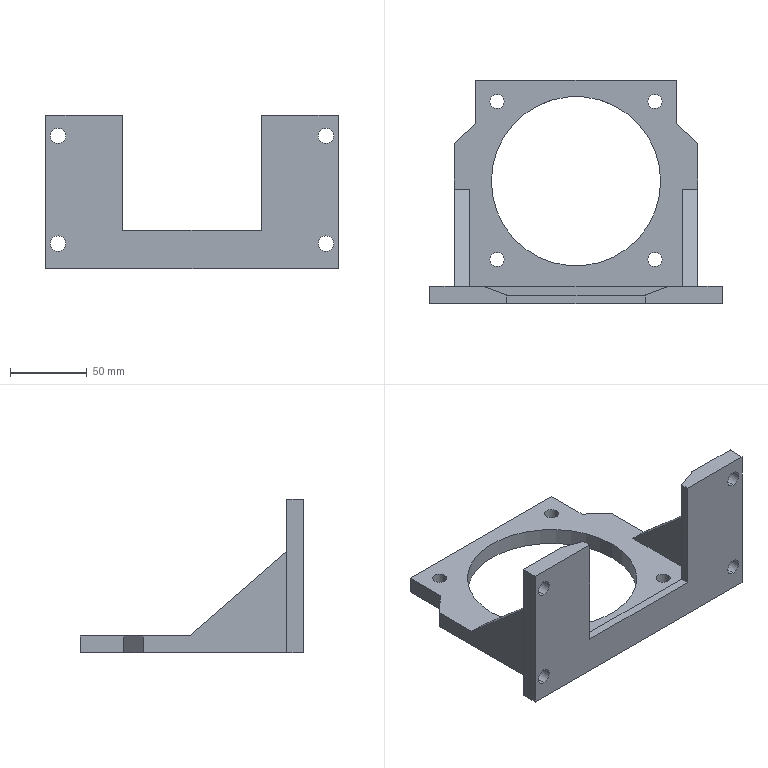Part | SolidWorks | features ICE 3, Extrusion 1, MirrorPattern 1 | 1 solid | 45 faces | box 190 x 145 x 100 mm | volume 268946 mm3 | plane 27 | cylinder 18 | commonest cylinder face diameters 9.2 x8 10 x8 110 x2
STEP:
#1=CARTESIAN_POINT('',(87.,-80.,85.957));
#2=VERTEX_POINT('',#1);
#3=CARTESIAN_POINT('',(87.,-80.,75.957));
#4=VERTEX_POINT('',#3);
#5=CARTESIAN_POINT('',(87.,-80.,80.957));
#6=DIRECTION('',(0.,-1.,0.));
#7=DIRECTION('',(0.,0.,1.));
#8=AXIS2_PLACEMENT_3D('',#5,#6,#7);
#9=CIRCLE('',#8,5.);
#10=EDGE_CURVE('',#2,#4,#9,.T.);
#11=ORIENTED_EDGE('',*,*,#10,.T.);
#12=CARTESIAN_POINT('',(87.,-69.,75.957));
#13=VERTEX_POINT('',#12);
#14=CARTESIAN_POINT('',(87.,-80.,75.957));
#15=DIRECTION('',(0.,1.,0.));
#16=VECTOR('',#15,1000.);
#17=LINE('',#14,#16);
#18=EDGE_CURVE('',#4,#13,#17,.T.);
#19=ORIENTED_EDGE('',*,*,#18,.T.);
#20=CARTESIAN_POINT('',(87.,-69.,85.957));
#21=VERTEX_POINT('',#20);
#22=CARTESIAN_POINT('',(87.,-69.,80.957));
#23=DIRECTION('',(0.,-1.,0.));
#24=DIRECTION('',(0.,0.,1.));
#25=AXIS2_PLACEMENT_3D('',#22,#23,#24);
#26=CIRCLE('',#25,5.);
#27=EDGE_CURVE('',#21,#13,#26,.T.);
#28=ORIENTED_EDGE('',*,*,#27,.F.);
#29=CARTESIAN_POINT('',(87.,-80.,85.957));
#30=DIRECTION('',(0.,1.,0.));
#31=VECTOR('',#30,1000.);
#32=LINE('',#29,#31);
#33=EDGE_CURVE('',#2,#21,#32,.T.);
#34=ORIENTED_EDGE('',*,*,#33,.F.);
#35=EDGE_LOOP('',(#11,#19,#28,#34));
#36=FACE_OUTER_BOUND('',#35,.T.);
#37=CARTESIAN_POINT('',(87.,-80.,80.957));
#38=DIRECTION('',(0.,1.,0.));
#39=DIRECTION('',(0.,0.,1.));
#40=AXIS2_PLACEMENT_3D('',#37,#38,#39);
#41=CYLINDRICAL_SURFACE('',#40,5.);
#42=ADVANCED_FACE('',(#36),#41,.F.);
#43=CARTESIAN_POINT('',(87.,-80.,15.957));
#44=VERTEX_POINT('',#43);
#45=CARTESIAN_POINT('',(87.,-80.,5.957));
#46=VERTEX_POINT('',#45);
#47=CARTESIAN_POINT('',(87.,-80.,10.957));
#48=DIRECTION('',(0.,-1.,0.));
#49=DIRECTION('',(0.,0.,1.));
#50=AXIS2_PLACEMENT_3D('',#47,#48,#49);
#51=CIRCLE('',#50,5.);
#52=EDGE_CURVE('',#44,#46,#51,.T.);
#53=ORIENTED_EDGE('',*,*,#52,.T.);
#54=CARTESIAN_POINT('',(87.,-69.,5.957));
#55=VERTEX_POINT('',#54);
#56=CARTESIAN_POINT('',(87.,-80.,5.957));
#57=DIRECTION('',(0.,1.,0.));
#58=VECTOR('',#57,1000.);
#59=LINE('',#56,#58);
#60=EDGE_CURVE('',#46,#55,#59,.T.);
#61=ORIENTED_EDGE('',*,*,#60,.T.);
#62=CARTESIAN_POINT('',(87.,-69.,15.957));
#63=VERTEX_POINT('',#62);
#64=CARTESIAN_POINT('',(87.,-69.,10.957));
#65=DIRECTION('',(0.,-1.,0.));
#66=DIRECTION('',(0.,0.,1.));
#67=AXIS2_PLACEMENT_3D('',#64,#65,#66);
#68=CIRCLE('',#67,5.);
#69=EDGE_CURVE('',#63,#55,#68,.T.);
#70=ORIENTED_EDGE('',*,*,#69,.F.);
#71=CARTESIAN_POINT('',(87.,-80.,15.957));
#72=DIRECTION('',(0.,1.,0.));
#73=VECTOR('',#72,1000.);
#74=LINE('',#71,#73);
#75=EDGE_CURVE('',#44,#63,#74,.T.);
#76=ORIENTED_EDGE('',*,*,#75,.F.);
#77=EDGE_LOOP('',(#53,#61,#70,#76));
#78=FACE_OUTER_BOUND('',#77,.T.);
#79=CARTESIAN_POINT('',(87.,-80.,10.957));
#80=DIRECTION('',(0.,1.,0.));
#81=DIRECTION('',(0.,0.,1.));
#82=AXIS2_PLACEMENT_3D('',#79,#80,#81);
#83=CYLINDRICAL_SURFACE('',#82,5.);
#84=ADVANCED_FACE('',(#78),#83,.F.);
#85=CARTESIAN_POINT('',(-87.,-80.,15.957));
#86=VERTEX_POINT('',#85);
#87=CARTESIAN_POINT('',(-87.,-80.,5.957));
#88=VERTEX_POINT('',#87);
#89=CARTESIAN_POINT('',(-87.,-80.,10.957));
#90=DIRECTION('',(0.,-1.,0.));
#91=DIRECTION('',(0.,0.,-1.));
#92=AXIS2_PLACEMENT_3D('',#89,#90,#91);
#93=CIRCLE('',#92,5.);
#94=EDGE_CURVE('',#86,#88,#93,.T.);
#95=ORIENTED_EDGE('',*,*,#94,.T.);
#96=CARTESIAN_POINT('',(-87.,-69.,5.957));
#97=VERTEX_POINT('',#96);
#98=CARTESIAN_POINT('',(-87.,-80.,5.957));
#99=DIRECTION('',(0.,1.,0.));
#100=VECTOR('',#99,1000.);
#101=LINE('',#98,#100);
#102=EDGE_CURVE('',#88,#97,#101,.T.);
#103=ORIENTED_EDGE('',*,*,#102,.T.);
#104=CARTESIAN_POINT('',(-87.,-69.,15.957));
#105=VERTEX_POINT('',#104);
#106=CARTESIAN_POINT('',(-87.,-69.,10.957));
#107=DIRECTION('',(0.,-1.,0.));
#108=DIRECTION('',(0.,0.,-1.));
#109=AXIS2_PLACEMENT_3D('',#106,#107,#108);
#110=CIRCLE('',#109,5.);
#111=EDGE_CURVE('',#105,#97,#110,.T.);
#112=ORIENTED_EDGE('',*,*,#111,.F.);
#113=CARTESIAN_POINT('',(-87.,-80.,15.957));
#114=DIRECTION('',(0.,1.,0.));
#115=VECTOR('',#114,1000.);
#116=LINE('',#113,#115);
#117=EDGE_CURVE('',#86,#105,#116,.T.);
#118=ORIENTED_EDGE('',*,*,#117,.F.);
#119=EDGE_LOOP('',(#95,#103,#112,#118));
#120=FACE_OUTER_BOUND('',#119,.T.);
#121=CARTESIAN_POINT('',(-87.,-80.,10.957));
#122=DIRECTION('',(0.,1.,0.));
#123=DIRECTION('',(0.,0.,1.));
#124=AXIS2_PLACEMENT_3D('',#121,#122,#123);
#125=CYLINDRICAL_SURFACE('',#124,5.);
#126=ADVANCED_FACE('',(#120),#125,.F.);
#127=CARTESIAN_POINT('',(-87.,-80.,85.957));
#128=VERTEX_POINT('',#127);
#129=CARTESIAN_POINT('',(-87.,-80.,75.957));
#130=VERTEX_POINT('',#129);
#131=CARTESIAN_POINT('',(-87.,-80.,80.957));
#132=DIRECTION('',(0.,-1.,0.));
#133=DIRECTION('',(0.,0.,-1.));
#134=AXIS2_PLACEMENT_3D('',#131,#132,#133);
#135=CIRCLE('',#134,5.);
#136=EDGE_CURVE('',#128,#130,#135,.T.);
#137=ORIENTED_EDGE('',*,*,#136,.T.);
#138=CARTESIAN_POINT('',(-87.,-69.,75.957));
#139=VERTEX_POINT('',#138);
#140=CARTESIAN_POINT('',(-87.,-80.,75.957));
#141=DIRECTION('',(0.,1.,0.));
#142=VECTOR('',#141,1000.);
#143=LINE('',#140,#142);
#144=EDGE_CURVE('',#130,#139,#143,.T.);
#145=ORIENTED_EDGE('',*,*,#144,.T.);
#146=CARTESIAN_POINT('',(-87.,-69.,85.957));
#147=VERTEX_POINT('',#146);
#148=CARTESIAN_POINT('',(-87.,-69.,80.957));
#149=DIRECTION('',(0.,-1.,0.));
#150=DIRECTION('',(0.,0.,-1.));
#151=AXIS2_PLACEMENT_3D('',#148,#149,#150);
#152=CIRCLE('',#151,5.);
#153=EDGE_CURVE('',#147,#139,#152,.T.);
#154=ORIENTED_EDGE('',*,*,#153,.F.);
#155=CARTESIAN_POINT('',(-87.,-80.,85.957));
#156=DIRECTION('',(0.,1.,0.));
#157=VECTOR('',#156,1000.);
#158=LINE('',#155,#157);
#159=EDGE_CURVE('',#128,#147,#158,.T.);
#160=ORIENTED_EDGE('',*,*,#159,.F.);
#161=EDGE_LOOP('',(#137,#145,#154,#160));
#162=FACE_OUTER_BOUND('',#161,.T.);
#163=CARTESIAN_POINT('',(-87.,-80.,80.957));
#164=DIRECTION('',(0.,1.,0.));
#165=DIRECTION('',(0.,0.,1.));
#166=AXIS2_PLACEMENT_3D('',#163,#164,#165);
#167=CYLINDRICAL_SURFACE('',#166,5.);
#168=ADVANCED_FACE('',(#162),#167,.F.);
#169=CARTESIAN_POINT('',(-46.7,-51.3,5.5));
#170=VERTEX_POINT('',#169);
#171=CARTESIAN_POINT('',(-55.9,-51.3,5.5));
#172=VERTEX_POINT('',#171);
#173=CARTESIAN_POINT('',(-51.3,-51.3,5.5));
#174=DIRECTION('',(0.,0.,-1.));
#175=DIRECTION('',(1.,0.,0.));
#176=AXIS2_PLACEMENT_3D('',#173,#174,#175);
#177=CIRCLE('',#176,4.6);
#178=EDGE_CURVE('',#170,#172,#177,.T.);
#179=ORIENTED_EDGE('',*,*,#178,.F.);
#180=CARTESIAN_POINT('',(-46.7,-51.3,-5.5));
#181=VERTEX_POINT('',#180);
#182=CARTESIAN_POINT('',(-46.7,-51.3,5.5));
#183=DIRECTION('',(0.,0.,-1.));
#184=VECTOR('',#183,1000.);
#185=LINE('',#182,#184);
#186=EDGE_CURVE('',#170,#181,#185,.T.);
#187=ORIENTED_EDGE('',*,*,#186,.T.);
#188=CARTESIAN_POINT('',(-55.9,-51.3,-5.5));
#189=VERTEX_POINT('',#188);
#190=CARTESIAN_POINT('',(-51.3,-51.3,-5.5));
#191=DIRECTION('',(0.,0.,-1.));
#192=DIRECTION('',(1.,0.,0.));
#193=AXIS2_PLACEMENT_3D('',#190,#191,#192);
#194=CIRCLE('',#193,4.6);
#195=EDGE_CURVE('',#181,#189,#194,.T.);
#196=ORIENTED_EDGE('',*,*,#195,.T.);
#197=CARTESIAN_POINT('',(-55.9,-51.3,5.5));
#198=DIRECTION('',(0.,0.,-1.));
#199=VECTOR('',#198,1000.);
#200=LINE('',#197,#199);
#201=EDGE_CURVE('',#172,#189,#200,.T.);
#202=ORIENTED_EDGE('',*,*,#201,.F.);
#203=EDGE_LOOP('',(#179,#187,#196,#202));
#204=FACE_OUTER_BOUND('',#203,.T.);
#205=CARTESIAN_POINT('',(-51.3,-51.3,5.5));
#206=DIRECTION('',(0.,0.,-1.));
#207=DIRECTION('',(-1.,0.,0.));
#208=AXIS2_PLACEMENT_3D('',#205,#206,#207);
#209=CYLINDRICAL_SURFACE('',#208,4.6);
#210=ADVANCED_FACE('',(#204),#209,.F.);
#211=CARTESIAN_POINT('',(55.9,-51.3,5.5));
#212=VERTEX_POINT('',#211);
#213=CARTESIAN_POINT('',(46.7,-51.3,5.5));
#214=VERTEX_POINT('',#213);
#215=CARTESIAN_POINT('',(51.3,-51.3,5.5));
#216=DIRECTION('',(0.,0.,-1.));
#217=DIRECTION('',(1.,0.,0.));
#218=AXIS2_PLACEMENT_3D('',#215,#216,#217);
#219=CIRCLE('',#218,4.6);
#220=EDGE_CURVE('',#212,#214,#219,.T.);
#221=ORIENTED_EDGE('',*,*,#220,.F.);
#222=CARTESIAN_POINT('',(55.9,-51.3,-5.5));
#223=VERTEX_POINT('',#222);
#224=CARTESIAN_POINT('',(55.9,-51.3,5.5));
#225=DIRECTION('',(0.,0.,-1.));
#226=VECTOR('',#225,1000.);
#227=LINE('',#224,#226);
#228=EDGE_CURVE('',#212,#223,#227,.T.);
#229=ORIENTED_EDGE('',*,*,#228,.T.);
#230=CARTESIAN_POINT('',(46.7,-51.3,-5.5));
#231=VERTEX_POINT('',#230);
#232=CARTESIAN_POINT('',(51.3,-51.3,-5.5));
#233=DIRECTION('',(0.,0.,-1.));
#234=DIRECTION('',(1.,0.,0.));
#235=AXIS2_PLACEMENT_3D('',#232,#233,#234);
#236=CIRCLE('',#235,4.6);
#237=EDGE_CURVE('',#223,#231,#236,.T.);
#238=ORIENTED_EDGE('',*,*,#237,.T.);
#239=CARTESIAN_POINT('',(46.7,-51.3,5.5));
#240=DIRECTION('',(0.,0.,-1.));
#241=VECTOR('',#240,1000.);
#242=LINE('',#239,#241);
#243=EDGE_CURVE('',#214,#231,#242,.T.);
#244=ORIENTED_EDGE('',*,*,#243,.F.);
#245=EDGE_LOOP('',(#221,#229,#238,#244));
#246=FACE_OUTER_BOUND('',#245,.T.);
#247=CARTESIAN_POINT('',(51.3,-51.3,5.5));
#248=DIRECTION('',(0.,0.,-1.));
#249=DIRECTION('',(-1.,0.,0.));
#250=AXIS2_PLACEMENT_3D('',#247,#248,#249);
#251=CYLINDRICAL_SURFACE('',#250,4.6);
#252=ADVANCED_FACE('',(#246),#251,.F.);
#253=CARTESIAN_POINT('',(46.7,51.3,5.5));
#254=VERTEX_POINT('',#253);
#255=CARTESIAN_POINT('',(55.9,51.3,5.5));
#256=VERTEX_POINT('',#255);
#257=CARTESIAN_POINT('',(51.3,51.3,5.5));
#258=DIRECTION('',(0.,0.,1.));
#259=DIRECTION('',(1.,0.,0.));
#260=AXIS2_PLACEMENT_3D('',#257,#258,#259);
#261=CIRCLE('',#260,4.6);
#262=EDGE_CURVE('',#254,#256,#261,.T.);
#263=ORIENTED_EDGE('',*,*,#262,.T.);
#264=CARTESIAN_POINT('',(55.9,51.3,-5.5));
#265=VERTEX_POINT('',#264);
#266=CARTESIAN_POINT('',(55.9,51.3,5.5));
#267=DIRECTION('',(0.,0.,-1.));
#268=VECTOR('',#267,1000.);
#269=LINE('',#266,#268);
#270=EDGE_CURVE('',#256,#265,#269,.T.);
#271=ORIENTED_EDGE('',*,*,#270,.T.);
#272=CARTESIAN_POINT('',(46.7,51.3,-5.5));
#273=VERTEX_POINT('',#272);
#274=CARTESIAN_POINT('',(51.3,51.3,-5.5));
#275=DIRECTION('',(0.,0.,1.));
#276=DIRECTION('',(1.,0.,0.));
#277=AXIS2_PLACEMENT_3D('',#274,#275,#276);
#278=CIRCLE('',#277,4.6);
#279=EDGE_CURVE('',#273,#265,#278,.T.);
#280=ORIENTED_EDGE('',*,*,#279,.F.);
#281=CARTESIAN_POINT('',(46.7,51.3,5.5));
#282=DIRECTION('',(0.,0.,-1.));
#283=VECTOR('',#282,1000.);
#284=LINE('',#281,#283);
#285=EDGE_CURVE('',#254,#273,#284,.T.);
#286=ORIENTED_EDGE('',*,*,#285,.F.);
#287=EDGE_LOOP('',(#263,#271,#280,#286));
#288=FACE_OUTER_BOUND('',#287,.T.);
#289=CARTESIAN_POINT('',(51.3,51.3,5.5));
#290=DIRECTION('',(0.,0.,-1.));
#291=DIRECTION('',(-1.,0.,0.));
#292=AXIS2_PLACEMENT_3D('',#289,#290,#291);
#293=CYLINDRICAL_SURFACE('',#292,4.6);
#294=ADVANCED_FACE('',(#288),#293,.F.);
#295=CARTESIAN_POINT('',(-55.9,51.3,5.5));
#296=VERTEX_POINT('',#295);
#297=CARTESIAN_POINT('',(-46.7,51.3,5.5));
#298=VERTEX_POINT('',#297);
#299=CARTESIAN_POINT('',(-51.3,51.3,5.5));
#300=DIRECTION('',(0.,0.,1.));
#301=DIRECTION('',(1.,0.,0.));
#302=AXIS2_PLACEMENT_3D('',#299,#300,#301);
#303=CIRCLE('',#302,4.6);
#304=EDGE_CURVE('',#296,#298,#303,.T.);
#305=ORIENTED_EDGE('',*,*,#304,.T.);
#306=CARTESIAN_POINT('',(-46.7,51.3,-5.5));
#307=VERTEX_POINT('',#306);
#308=CARTESIAN_POINT('',(-46.7,51.3,5.5));
#309=DIRECTION('',(0.,0.,-1.));
#310=VECTOR('',#309,1000.);
#311=LINE('',#308,#310);
#312=EDGE_CURVE('',#298,#307,#311,.T.);
#313=ORIENTED_EDGE('',*,*,#312,.T.);
#314=CARTESIAN_POINT('',(-55.9,51.3,-5.5));
#315=VERTEX_POINT('',#314);
#316=CARTESIAN_POINT('',(-51.3,51.3,-5.5));
#317=DIRECTION('',(0.,0.,1.));
#318=DIRECTION('',(1.,0.,0.));
#319=AXIS2_PLACEMENT_3D('',#316,#317,#318);
#320=CIRCLE('',#319,4.6);
#321=EDGE_CURVE('',#315,#307,#320,.T.);
#322=ORIENTED_EDGE('',*,*,#321,.F.);
#323=CARTESIAN_POINT('',(-55.9,51.3,5.5));
#324=DIRECTION('',(0.,0.,-1.));
#325=VECTOR('',#324,1000.);
#326=LINE('',#323,#325);
#327=EDGE_CURVE('',#296,#315,#326,.T.);
#328=ORIENTED_EDGE('',*,*,#327,.F.);
#329=EDGE_LOOP('',(#305,#313,#322,#328));
#330=FACE_OUTER_BOUND('',#329,.T.);
#331=CARTESIAN_POINT('',(-51.3,51.3,5.5));
#332=DIRECTION('',(0.,0.,-1.));
#333=DIRECTION('',(-1.,0.,0.));
#334=AXIS2_PLACEMENT_3D('',#331,#332,#333);
#335=CYLINDRICAL_SURFACE('',#334,4.6);
#336=ADVANCED_FACE('',(#330),#335,.F.);
#337=CARTESIAN_POINT('',(-55.,-0.5,5.5));
#338=VERTEX_POINT('',#337);
#339=CARTESIAN_POINT('',(55.,-0.5,5.5));
#340=VERTEX_POINT('',#339);
#341=CARTESIAN_POINT('',(0.,-0.5,5.5));
#342=DIRECTION('',(0.,0.,1.));
#343=DIRECTION('',(1.,0.,0.));
#344=AXIS2_PLACEMENT_3D('',#341,#342,#343);
#345=CIRCLE('',#344,55.);
#346=EDGE_CURVE('',#338,#340,#345,.T.);
#347=ORIENTED_EDGE('',*,*,#346,.T.);
#348=CARTESIAN_POINT('',(55.,-0.5,-5.5));
#349=VERTEX_POINT('',#348);
#350=CARTESIAN_POINT('',(55.,-0.5,5.5));
#351=DIRECTION('',(0.,0.,-1.));
#352=VECTOR('',#351,1000.);
#353=LINE('',#350,#352);
#354=EDGE_CURVE('',#340,#349,#353,.T.);
#355=ORIENTED_EDGE('',*,*,#354,.T.);
#356=CARTESIAN_POINT('',(-55.,-0.5,-5.5));
#357=VERTEX_POINT('',#356);
#358=CARTESIAN_POINT('',(0.,-0.5,-5.5));
#359=DIRECTION('',(0.,0.,1.));
#360=DIRECTION('',(1.,0.,0.));
#361=AXIS2_PLACEMENT_3D('',#358,#359,#360);
#362=CIRCLE('',#361,55.);
#363=EDGE_CURVE('',#357,#349,#362,.T.);
#364=ORIENTED_EDGE('',*,*,#363,.F.);
#365=CARTESIAN_POINT('',(-55.,-0.5,5.5));
#366=DIRECTION('',(0.,0.,-1.));
#367=VECTOR('',#366,1000.);
#368=LINE('',#365,#367);
#369=EDGE_CURVE('',#338,#357,#368,.T.);
#370=ORIENTED_EDGE('',*,*,#369,.F.);
#371=EDGE_LOOP('',(#347,#355,#364,#370));
#372=FACE_OUTER_BOUND('',#371,.T.);
#373=CARTESIAN_POINT('',(0.,-0.5,5.5));
#374=DIRECTION('',(0.,0.,-1.));
#375=DIRECTION('',(-1.,0.,0.));
#376=AXIS2_PLACEMENT_3D('',#373,#374,#375);
#377=CYLINDRICAL_SURFACE('',#376,55.);
#378=ADVANCED_FACE('',(#372),#377,.F.);
#379=CARTESIAN_POINT('',(-79.,-5.675,5.5));
#380=VERTEX_POINT('',#379);
#381=CARTESIAN_POINT('',(-69.,-5.675,5.5));
#382=VERTEX_POINT('',#381);
#383=CARTESIAN_POINT('',(-79.,-5.675,5.5));
#384=DIRECTION('',(1.,0.,0.));
#385=VECTOR('',#384,1000.);
#386=LINE('',#383,#385);
#387=EDGE_CURVE('',#380,#382,#386,.T.);
#388=ORIENTED_EDGE('',*,*,#387,.T.);
#389=CARTESIAN_POINT('',(-69.,-69.,5.5));
#390=VERTEX_POINT('',#389);
#391=CARTESIAN_POINT('',(-69.,-69.,5.5));
#392=DIRECTION('',(0.,1.,0.));
#393=VECTOR('',#392,1000.);
#394=LINE('',#391,#393);
#395=EDGE_CURVE('',#390,#382,#394,.T.);
#396=ORIENTED_EDGE('',*,*,#395,.F.);
#397=CARTESIAN_POINT('',(69.,-69.,5.5));
#398=VERTEX_POINT('',#397);
#399=CARTESIAN_POINT('',(0.,-69.,5.5));
#400=DIRECTION('',(-1.,0.,0.));
#401=VECTOR('',#400,1000.);
#402=LINE('',#399,#401);
#403=EDGE_CURVE('',#398,#390,#402,.T.);
#404=ORIENTED_EDGE('',*,*,#403,.F.);
#405=CARTESIAN_POINT('',(69.,-5.675,5.5));
#406=VERTEX_POINT('',#405);
#407=CARTESIAN_POINT('',(69.,-69.,5.5));
#408=DIRECTION('',(0.,1.,0.));
#409=VECTOR('',#408,1000.);
#410=LINE('',#407,#409);
#411=EDGE_CURVE('',#398,#406,#410,.T.);
#412=ORIENTED_EDGE('',*,*,#411,.T.);
#413=CARTESIAN_POINT('',(79.,-5.675,5.5));
#414=VERTEX_POINT('',#413);
#415=CARTESIAN_POINT('',(79.,-5.675,5.5));
#416=DIRECTION('',(-1.,0.,0.));
#417=VECTOR('',#416,1000.);
#418=LINE('',#415,#417);
#419=EDGE_CURVE('',#414,#406,#418,.T.);
#420=ORIENTED_EDGE('',*,*,#419,.F.);
#421=CARTESIAN_POINT('',(79.,24.101,5.5));
#422=VERTEX_POINT('',#421);
#423=CARTESIAN_POINT('',(79.,0.,5.5));
#424=DIRECTION('',(0.,-1.,0.));
#425=VECTOR('',#424,1000.);
#426=LINE('',#423,#425);
#427=EDGE_CURVE('',#422,#414,#426,.T.);
#428=ORIENTED_EDGE('',*,*,#427,.F.);
#429=CARTESIAN_POINT('',(65.,36.95,5.5));
#430=VERTEX_POINT('',#429);
#431=CARTESIAN_POINT('',(48.127,52.437,5.5));
#432=DIRECTION('',(0.7367,-0.6762,0.));
#433=VECTOR('',#432,1000.);
#434=LINE('',#431,#433);
#435=EDGE_CURVE('',#430,#422,#434,.T.);
#436=ORIENTED_EDGE('',*,*,#435,.F.);
#437=CARTESIAN_POINT('',(65.,65.,5.5));
#438=VERTEX_POINT('',#437);
#439=CARTESIAN_POINT('',(65.,0.,5.5));
#440=DIRECTION('',(0.,1.,0.));
#441=VECTOR('',#440,1000.);
#442=LINE('',#439,#441);
#443=EDGE_CURVE('',#430,#438,#442,.T.);
#444=ORIENTED_EDGE('',*,*,#443,.T.);
#445=CARTESIAN_POINT('',(-65.,65.,5.5));
#446=VERTEX_POINT('',#445);
#447=CARTESIAN_POINT('',(0.,65.,5.5));
#448=DIRECTION('',(-1.,0.,0.));
#449=VECTOR('',#448,1000.);
#450=LINE('',#447,#449);
#451=EDGE_CURVE('',#438,#446,#450,.T.);
#452=ORIENTED_EDGE('',*,*,#451,.T.);
#453=CARTESIAN_POINT('',(-65.,36.95,5.5));
#454=VERTEX_POINT('',#453);
#455=CARTESIAN_POINT('',(-65.,0.,5.5));
#456=DIRECTION('',(0.,1.,0.));
#457=VECTOR('',#456,1000.);
#458=LINE('',#455,#457);
#459=EDGE_CURVE('',#454,#446,#458,.T.);
#460=ORIENTED_EDGE('',*,*,#459,.F.);
#461=CARTESIAN_POINT('',(-79.,24.101,5.5));
#462=VERTEX_POINT('',#461);
#463=CARTESIAN_POINT('',(-48.127,52.437,5.5));
#464=DIRECTION('',(-0.7367,-0.6762,0.));
#465=VECTOR('',#464,1000.);
#466=LINE('',#463,#465);
#467=EDGE_CURVE('',#454,#462,#466,.T.);
#468=ORIENTED_EDGE('',*,*,#467,.T.);
#469=CARTESIAN_POINT('',(-79.,0.,5.5));
#470=DIRECTION('',(0.,-1.,0.));
#471=VECTOR('',#470,1000.);
#472=LINE('',#469,#471);
#473=EDGE_CURVE('',#462,#380,#472,.T.);
#474=ORIENTED_EDGE('',*,*,#473,.T.);
#475=EDGE_LOOP('',(#388,#396,#404,#412,#420,#428,#436,#444,#452,#460,#468,#474));
#476=FACE_OUTER_BOUND('',#475,.T.);
#477=CARTESIAN_POINT('',(51.3,-51.3,5.5));
#478=DIRECTION('',(0.,0.,-1.));
#479=DIRECTION('',(1.,0.,0.));
#480=AXIS2_PLACEMENT_3D('',#477,#478,#479);
#481=CIRCLE('',#480,4.6);
#482=EDGE_CURVE('',#214,#212,#481,.T.);
#483=ORIENTED_EDGE('',*,*,#482,.T.);
#484=ORIENTED_EDGE('',*,*,#220,.T.);
#485=EDGE_LOOP('',(#483,#484));
#486=FACE_BOUND('',#485,.T.);
#487=ORIENTED_EDGE('',*,*,#262,.F.);
#488=CARTESIAN_POINT('',(51.3,51.3,5.5));
#489=DIRECTION('',(0.,0.,1.));
#490=DIRECTION('',(1.,0.,0.));
#491=AXIS2_PLACEMENT_3D('',#488,#489,#490);
#492=CIRCLE('',#491,4.6);
#493=EDGE_CURVE('',#256,#254,#492,.T.);
#494=ORIENTED_EDGE('',*,*,#493,.F.);
#495=EDGE_LOOP('',(#487,#494));
#496=FACE_BOUND('',#495,.T.);
#497=ORIENTED_EDGE('',*,*,#304,.F.);
#498=CARTESIAN_POINT('',(-51.3,51.3,5.5));
#499=DIRECTION('',(0.,0.,1.));
#500=DIRECTION('',(1.,0.,0.));
#501=AXIS2_PLACEMENT_3D('',#498,#499,#500);
#502=CIRCLE('',#501,4.6);
#503=EDGE_CURVE('',#298,#296,#502,.T.);
#504=ORIENTED_EDGE('',*,*,#503,.F.);
#505=EDGE_LOOP('',(#497,#504));
#506=FACE_BOUND('',#505,.T.);
#507=ORIENTED_EDGE('',*,*,#346,.F.);
#508=CARTESIAN_POINT('',(0.,-0.5,5.5));
#509=DIRECTION('',(0.,0.,1.));
#510=DIRECTION('',(1.,0.,0.));
#511=AXIS2_PLACEMENT_3D('',#508,#509,#510);
#512=CIRCLE('',#511,55.);
#513=EDGE_CURVE('',#340,#338,#512,.T.);
#514=ORIENTED_EDGE('',*,*,#513,.F.);
#515=EDGE_LOOP('',(#507,#514));
#516=FACE_BOUND('',#515,.T.);
#517=CARTESIAN_POINT('',(-51.3,-51.3,5.5));
#518=DIRECTION('',(0.,0.,-1.));
#519=DIRECTION('',(1.,0.,0.));
#520=AXIS2_PLACEMENT_3D('',#517,#518,#519);
#521=CIRCLE('',#520,4.6);
#522=EDGE_CURVE('',#172,#170,#521,.T.);
#523=ORIENTED_EDGE('',*,*,#522,.T.);
#524=ORIENTED_EDGE('',*,*,#178,.T.);
#525=EDGE_LOOP('',(#523,#524));
#526=FACE_BOUND('',#525,.T.);
#527=CARTESIAN_POINT('',(0.,0.,5.5));
#528=DIRECTION('',(0.,0.,1.));
#529=DIRECTION('',(1.,0.,0.));
#530=AXIS2_PLACEMENT_3D('',#527,#528,#529);
#531=PLANE('',#530);
#532=ADVANCED_FACE('',(#476,#486,#496,#506,#516,#526),#531,.T.);
#533=CARTESIAN_POINT('',(-79.,24.101,-5.5));
#534=VERTEX_POINT('',#533);
#535=CARTESIAN_POINT('',(-79.,-69.,-5.5));
#536=VERTEX_POINT('',#535);
#537=CARTESIAN_POINT('',(-79.,0.,-5.5));
#538=DIRECTION('',(0.,-1.,0.));
#539=VECTOR('',#538,1000.);
#540=LINE('',#537,#539);
#541=EDGE_CURVE('',#534,#536,#540,.T.);
#542=ORIENTED_EDGE('',*,*,#541,.T.);
#543=CARTESIAN_POINT('',(-79.,-69.,60.457));
#544=VERTEX_POINT('',#543);
#545=CARTESIAN_POINT('',(-79.,-69.,5.5));
#546=DIRECTION('',(0.,0.,-1.));
#547=VECTOR('',#546,1000.);
#548=LINE('',#545,#547);
#549=EDGE_CURVE('',#544,#536,#548,.T.);
#550=ORIENTED_EDGE('',*,*,#549,.F.);
#551=CARTESIAN_POINT('',(-79.,-5.675,5.5));
#552=DIRECTION('',(0.,-0.7552,0.6554));
#553=VECTOR('',#552,1000.);
#554=LINE('',#551,#553);
#555=EDGE_CURVE('',#380,#544,#554,.T.);
#556=ORIENTED_EDGE('',*,*,#555,.F.);
#557=ORIENTED_EDGE('',*,*,#473,.F.);
#558=CARTESIAN_POINT('',(-79.,24.101,5.5));
#559=DIRECTION('',(0.,0.,-1.));
#560=VECTOR('',#559,1000.);
#561=LINE('',#558,#560);
#562=EDGE_CURVE('',#462,#534,#561,.T.);
#563=ORIENTED_EDGE('',*,*,#562,.T.);
#564=EDGE_LOOP('',(#542,#550,#556,#557,#563));
#565=FACE_OUTER_BOUND('',#564,.T.);
#566=CARTESIAN_POINT('',(-79.,0.,5.5));
#567=DIRECTION('',(1.,0.,0.));
#568=DIRECTION('',(0.,0.,-1.));
#569=AXIS2_PLACEMENT_3D('',#566,#567,#568);
#570=PLANE('',#569);
#571=ADVANCED_FACE('',(#565),#570,.F.);
#572=CARTESIAN_POINT('',(79.,24.101,-5.5));
#573=VERTEX_POINT('',#572);
#574=CARTESIAN_POINT('',(79.,-69.,-5.5));
#575=VERTEX_POINT('',#574);
#576=CARTESIAN_POINT('',(79.,0.,-5.5));
#577=DIRECTION('',(0.,-1.,0.));
#578=VECTOR('',#577,1000.);
#579=LINE('',#576,#578);
#580=EDGE_CURVE('',#573,#575,#579,.T.);
#581=ORIENTED_EDGE('',*,*,#580,.F.);
#582=CARTESIAN_POINT('',(79.,24.101,5.5));
#583=DIRECTION('',(0.,0.,-1.));
#584=VECTOR('',#583,1000.);
#585=LINE('',#582,#584);
#586=EDGE_CURVE('',#422,#573,#585,.T.);
#587=ORIENTED_EDGE('',*,*,#586,.F.);
#588=ORIENTED_EDGE('',*,*,#427,.T.);
#589=CARTESIAN_POINT('',(79.,-69.,60.457));
#590=VERTEX_POINT('',#589);
#591=CARTESIAN_POINT('',(79.,-5.675,5.5));
#592=DIRECTION('',(0.,-0.7552,0.6554));
#593=VECTOR('',#592,1000.);
#594=LINE('',#591,#593);
#595=EDGE_CURVE('',#414,#590,#594,.T.);
#596=ORIENTED_EDGE('',*,*,#595,.T.);
#597=CARTESIAN_POINT('',(79.,-69.,5.5));
#598=DIRECTION('',(0.,0.,-1.));
#599=VECTOR('',#598,1000.);
#600=LINE('',#597,#599);
#601=EDGE_CURVE('',#590,#575,#600,.T.);
#602=ORIENTED_EDGE('',*,*,#601,.T.);
#603=EDGE_LOOP('',(#581,#587,#588,#596,#602));
#604=FACE_OUTER_BOUND('',#603,.T.);
#605=CARTESIAN_POINT('',(79.,0.,5.5));
#606=DIRECTION('',(1.,0.,0.));
#607=DIRECTION('',(0.,1.,0.));
#608=AXIS2_PLACEMENT_3D('',#605,#606,#607);
#609=PLANE('',#608);
#610=ADVANCED_FACE('',(#604),#609,.T.);
#611=CARTESIAN_POINT('',(65.,36.95,-5.5));
#612=VERTEX_POINT('',#611);
#613=CARTESIAN_POINT('',(48.127,52.437,-5.5));
#614=DIRECTION('',(0.7367,-0.6762,0.));
#615=VECTOR('',#614,1000.);
#616=LINE('',#613,#615);
#617=EDGE_CURVE('',#612,#573,#616,.T.);
#618=ORIENTED_EDGE('',*,*,#617,.F.);
#619=CARTESIAN_POINT('',(65.,36.95,5.5));
#620=DIRECTION('',(0.,0.,-1.));
#621=VECTOR('',#620,1000.);
#622=LINE('',#619,#621);
#623=EDGE_CURVE('',#430,#612,#622,.T.);
#624=ORIENTED_EDGE('',*,*,#623,.F.);
#625=ORIENTED_EDGE('',*,*,#435,.T.);
#626=ORIENTED_EDGE('',*,*,#586,.T.);
#627=EDGE_LOOP('',(#618,#624,#625,#626));
#628=FACE_OUTER_BOUND('',#627,.T.);
#629=CARTESIAN_POINT('',(48.127,52.437,5.5));
#630=DIRECTION('',(0.6762,0.7367,0.));
#631=DIRECTION('',(-0.7367,0.6762,0.));
#632=AXIS2_PLACEMENT_3D('',#629,#630,#631);
#633=PLANE('',#632);
#634=ADVANCED_FACE('',(#628),#633,.T.);
#635=CARTESIAN_POINT('',(65.,65.,-5.5));
#636=VERTEX_POINT('',#635);
#637=CARTESIAN_POINT('',(65.,0.,-5.5));
#638=DIRECTION('',(0.,1.,0.));
#639=VECTOR('',#638,1000.);
#640=LINE('',#637,#639);
#641=EDGE_CURVE('',#612,#636,#640,.T.);
#642=ORIENTED_EDGE('',*,*,#641,.T.);
#643=CARTESIAN_POINT('',(65.,65.,5.5));
#644=DIRECTION('',(0.,0.,-1.));
#645=VECTOR('',#644,1000.);
#646=LINE('',#643,#645);
#647=EDGE_CURVE('',#438,#636,#646,.T.);
#648=ORIENTED_EDGE('',*,*,#647,.F.);
#649=ORIENTED_EDGE('',*,*,#443,.F.);
#650=ORIENTED_EDGE('',*,*,#623,.T.);
#651=EDGE_LOOP('',(#642,#648,#649,#650));
#652=FACE_OUTER_BOUND('',#651,.T.);
#653=CARTESIAN_POINT('',(65.,0.,5.5));
#654=DIRECTION('',(-1.,0.,0.));
#655=DIRECTION('',(0.,0.,1.));
#656=AXIS2_PLACEMENT_3D('',#653,#654,#655);
#657=PLANE('',#656);
#658=ADVANCED_FACE('',(#652),#657,.F.);
#659=CARTESIAN_POINT('',(-65.,65.,-5.5));
#660=VERTEX_POINT('',#659);
#661=CARTESIAN_POINT('',(0.,65.,-5.5));
#662=DIRECTION('',(-1.,0.,0.));
#663=VECTOR('',#662,1000.);
#664=LINE('',#661,#663);
#665=EDGE_CURVE('',#636,#660,#664,.T.);
#666=ORIENTED_EDGE('',*,*,#665,.T.);
#667=CARTESIAN_POINT('',(-65.,65.,5.5));
#668=DIRECTION('',(0.,0.,-1.));
#669=VECTOR('',#668,1000.);
#670=LINE('',#667,#669);
#671=EDGE_CURVE('',#446,#660,#670,.T.);
#672=ORIENTED_EDGE('',*,*,#671,.F.);
#673=ORIENTED_EDGE('',*,*,#451,.F.);
#674=ORIENTED_EDGE('',*,*,#647,.T.);
#675=EDGE_LOOP('',(#666,#672,#673,#674));
#676=FACE_OUTER_BOUND('',#675,.T.);
#677=CARTESIAN_POINT('',(0.,65.,5.5));
#678=DIRECTION('',(0.,-1.,0.));
#679=DIRECTION('',(1.,0.,0.));
#680=AXIS2_PLACEMENT_3D('',#677,#678,#679);
#681=PLANE('',#680);
#682=ADVANCED_FACE('',(#676),#681,.F.);
#683=CARTESIAN_POINT('',(-65.,36.95,-5.5));
#684=VERTEX_POINT('',#683);
#685=CARTESIAN_POINT('',(-65.,0.,-5.5));
#686=DIRECTION('',(0.,1.,0.));
#687=VECTOR('',#686,1000.);
#688=LINE('',#685,#687);
#689=EDGE_CURVE('',#684,#660,#688,.T.);
#690=ORIENTED_EDGE('',*,*,#689,.F.);
#691=CARTESIAN_POINT('',(-65.,36.95,5.5));
#692=DIRECTION('',(0.,0.,-1.));
#693=VECTOR('',#692,1000.);
#694=LINE('',#691,#693);
#695=EDGE_CURVE('',#454,#684,#694,.T.);
#696=ORIENTED_EDGE('',*,*,#695,.F.);
#697=ORIENTED_EDGE('',*,*,#459,.T.);
#698=ORIENTED_EDGE('',*,*,#671,.T.);
#699=EDGE_LOOP('',(#690,#696,#697,#698));
#700=FACE_OUTER_BOUND('',#699,.T.);
#701=CARTESIAN_POINT('',(-65.,0.,5.5));
#702=DIRECTION('',(-1.,0.,0.));
#703=DIRECTION('',(0.,0.,1.));
#704=AXIS2_PLACEMENT_3D('',#701,#702,#703);
#705=PLANE('',#704);
#706=ADVANCED_FACE('',(#700),#705,.T.);
#707=ORIENTED_EDGE('',*,*,#354,.F.);
#708=ORIENTED_EDGE('',*,*,#513,.T.);
#709=ORIENTED_EDGE('',*,*,#369,.T.);
#710=CARTESIAN_POINT('',(0.,-0.5,-5.5));
#711=DIRECTION('',(0.,0.,1.));
#712=DIRECTION('',(1.,0.,0.));
#713=AXIS2_PLACEMENT_3D('',#710,#711,#712);
#714=CIRCLE('',#713,55.);
#715=EDGE_CURVE('',#349,#357,#714,.T.);
#716=ORIENTED_EDGE('',*,*,#715,.F.);
#717=EDGE_LOOP('',(#707,#708,#709,#716));
#718=FACE_OUTER_BOUND('',#717,.T.);
#719=CARTESIAN_POINT('',(0.,-0.5,5.5));
#720=DIRECTION('',(0.,0.,-1.));
#721=DIRECTION('',(-1.,0.,0.));
#722=AXIS2_PLACEMENT_3D('',#719,#720,#721);
#723=CYLINDRICAL_SURFACE('',#722,55.);
#724=ADVANCED_FACE('',(#718),#723,.F.);
#725=ORIENTED_EDGE('',*,*,#312,.F.);
#726=ORIENTED_EDGE('',*,*,#503,.T.);
#727=ORIENTED_EDGE('',*,*,#327,.T.);
#728=CARTESIAN_POINT('',(-51.3,51.3,-5.5));
#729=DIRECTION('',(0.,0.,1.));
#730=DIRECTION('',(1.,0.,0.));
#731=AXIS2_PLACEMENT_3D('',#728,#729,#730);
#732=CIRCLE('',#731,4.6);
#733=EDGE_CURVE('',#307,#315,#732,.T.);
#734=ORIENTED_EDGE('',*,*,#733,.F.);
#735=EDGE_LOOP('',(#725,#726,#727,#734));
#736=FACE_OUTER_BOUND('',#735,.T.);
#737=CARTESIAN_POINT('',(-51.3,51.3,5.5));
#738=DIRECTION('',(0.,0.,-1.));
#739=DIRECTION('',(-1.,0.,0.));
#740=AXIS2_PLACEMENT_3D('',#737,#738,#739);
#741=CYLINDRICAL_SURFACE('',#740,4.6);
#742=ADVANCED_FACE('',(#736),#741,.F.);
#743=ORIENTED_EDGE('',*,*,#270,.F.);
#744=ORIENTED_EDGE('',*,*,#493,.T.);
#745=ORIENTED_EDGE('',*,*,#285,.T.);
#746=CARTESIAN_POINT('',(51.3,51.3,-5.5));
#747=DIRECTION('',(0.,0.,1.));
#748=DIRECTION('',(1.,0.,0.));
#749=AXIS2_PLACEMENT_3D('',#746,#747,#748);
#750=CIRCLE('',#749,4.6);
#751=EDGE_CURVE('',#265,#273,#750,.T.);
#752=ORIENTED_EDGE('',*,*,#751,.F.);
#753=EDGE_LOOP('',(#743,#744,#745,#752));
#754=FACE_OUTER_BOUND('',#753,.T.);
#755=CARTESIAN_POINT('',(51.3,51.3,5.5));
#756=DIRECTION('',(0.,0.,-1.));
#757=DIRECTION('',(-1.,0.,0.));
#758=AXIS2_PLACEMENT_3D('',#755,#756,#757);
#759=CYLINDRICAL_SURFACE('',#758,4.6);
#760=ADVANCED_FACE('',(#754),#759,.F.);
#761=ORIENTED_EDGE('',*,*,#228,.F.);
#762=ORIENTED_EDGE('',*,*,#482,.F.);
#763=ORIENTED_EDGE('',*,*,#243,.T.);
#764=CARTESIAN_POINT('',(51.3,-51.3,-5.5));
#765=DIRECTION('',(0.,0.,-1.));
#766=DIRECTION('',(1.,0.,0.));
#767=AXIS2_PLACEMENT_3D('',#764,#765,#766);
#768=CIRCLE('',#767,4.6);
#769=EDGE_CURVE('',#231,#223,#768,.T.);
#770=ORIENTED_EDGE('',*,*,#769,.T.);
#771=EDGE_LOOP('',(#761,#762,#763,#770));
#772=FACE_OUTER_BOUND('',#771,.T.);
#773=CARTESIAN_POINT('',(51.3,-51.3,5.5));
#774=DIRECTION('',(0.,0.,-1.));
#775=DIRECTION('',(-1.,0.,0.));
#776=AXIS2_PLACEMENT_3D('',#773,#774,#775);
#777=CYLINDRICAL_SURFACE('',#776,4.6);
#778=ADVANCED_FACE('',(#772),#777,.F.);
#779=CARTESIAN_POINT('',(-48.127,52.437,-5.5));
#780=DIRECTION('',(-0.7367,-0.6762,0.));
#781=VECTOR('',#780,1000.);
#782=LINE('',#779,#781);
#783=EDGE_CURVE('',#684,#534,#782,.T.);
#784=ORIENTED_EDGE('',*,*,#783,.T.);
#785=ORIENTED_EDGE('',*,*,#562,.F.);
#786=ORIENTED_EDGE('',*,*,#467,.F.);
#787=ORIENTED_EDGE('',*,*,#695,.T.);
#788=EDGE_LOOP('',(#784,#785,#786,#787));
#789=FACE_OUTER_BOUND('',#788,.T.);
#790=CARTESIAN_POINT('',(-48.127,52.437,5.5));
#791=DIRECTION('',(0.6762,-0.7367,0.));
#792=DIRECTION('',(0.7367,0.6762,0.));
#793=AXIS2_PLACEMENT_3D('',#790,#791,#792);
#794=PLANE('',#793);
#795=ADVANCED_FACE('',(#789),#794,.F.);
#796=ORIENTED_EDGE('',*,*,#186,.F.);
#797=ORIENTED_EDGE('',*,*,#522,.F.);
#798=ORIENTED_EDGE('',*,*,#201,.T.);
#799=CARTESIAN_POINT('',(-51.3,-51.3,-5.5));
#800=DIRECTION('',(0.,0.,-1.));
#801=DIRECTION('',(1.,0.,0.));
#802=AXIS2_PLACEMENT_3D('',#799,#800,#801);
#803=CIRCLE('',#802,4.6);
#804=EDGE_CURVE('',#189,#181,#803,.T.);
#805=ORIENTED_EDGE('',*,*,#804,.T.);
#806=EDGE_LOOP('',(#796,#797,#798,#805));
#807=FACE_OUTER_BOUND('',#806,.T.);
#808=CARTESIAN_POINT('',(-51.3,-51.3,5.5));
#809=DIRECTION('',(0.,0.,-1.));
#810=DIRECTION('',(-1.,0.,0.));
#811=AXIS2_PLACEMENT_3D('',#808,#809,#810);
#812=CYLINDRICAL_SURFACE('',#811,4.6);
#813=ADVANCED_FACE('',(#807),#812,.F.);
#814=ORIENTED_EDGE('',*,*,#541,.F.);
#815=ORIENTED_EDGE('',*,*,#783,.F.);
#816=ORIENTED_EDGE('',*,*,#689,.T.);
#817=ORIENTED_EDGE('',*,*,#665,.F.);
#818=ORIENTED_EDGE('',*,*,#641,.F.);
#819=ORIENTED_EDGE('',*,*,#617,.T.);
#820=ORIENTED_EDGE('',*,*,#580,.T.);
#821=CARTESIAN_POINT('',(0.,-69.,-5.5));
#822=DIRECTION('',(-1.,0.,0.));
#823=VECTOR('',#822,1000.);
#824=LINE('',#821,#823);
#825=EDGE_CURVE('',#575,#536,#824,.T.);
#826=ORIENTED_EDGE('',*,*,#825,.T.);
#827=EDGE_LOOP('',(#814,#815,#816,#817,#818,#819,#820,#826));
#828=FACE_OUTER_BOUND('',#827,.T.);
#829=ORIENTED_EDGE('',*,*,#769,.F.);
#830=ORIENTED_EDGE('',*,*,#237,.F.);
#831=EDGE_LOOP('',(#829,#830));
#832=FACE_BOUND('',#831,.T.);
#833=ORIENTED_EDGE('',*,*,#279,.T.);
#834=ORIENTED_EDGE('',*,*,#751,.T.);
#835=EDGE_LOOP('',(#833,#834));
#836=FACE_BOUND('',#835,.T.);
#837=ORIENTED_EDGE('',*,*,#321,.T.);
#838=ORIENTED_EDGE('',*,*,#733,.T.);
#839=EDGE_LOOP('',(#837,#838));
#840=FACE_BOUND('',#839,.T.);
#841=ORIENTED_EDGE('',*,*,#363,.T.);
#842=ORIENTED_EDGE('',*,*,#715,.T.);
#843=EDGE_LOOP('',(#841,#842));
#844=FACE_BOUND('',#843,.T.);
#845=ORIENTED_EDGE('',*,*,#804,.F.);
#846=ORIENTED_EDGE('',*,*,#195,.F.);
#847=EDGE_LOOP('',(#845,#846));
#848=FACE_BOUND('',#847,.T.);
#849=CARTESIAN_POINT('',(0.,0.,-5.5));
#850=DIRECTION('',(0.,0.,1.));
#851=DIRECTION('',(1.,0.,0.));
#852=AXIS2_PLACEMENT_3D('',#849,#850,#851);
#853=PLANE('',#852);
#854=ADVANCED_FACE('',(#828,#832,#836,#840,#844,#848),#853,.F.);
#855=CARTESIAN_POINT('',(-95.,-80.,94.457));
#856=VERTEX_POINT('',#855);
#857=CARTESIAN_POINT('',(-95.,-80.,-5.543));
#858=VERTEX_POINT('',#857);
#859=CARTESIAN_POINT('',(-95.,-80.,-5.543));
#860=DIRECTION('',(0.,0.,-1.));
#861=VECTOR('',#860,1000.);
#862=LINE('',#859,#861);
#863=EDGE_CURVE('',#856,#858,#862,.T.);
#864=ORIENTED_EDGE('',*,*,#863,.T.);
#865=CARTESIAN_POINT('',(95.,-80.,-5.543));
#866=VERTEX_POINT('',#865);
#867=CARTESIAN_POINT('',(-95.,-80.,-5.543));
#868=DIRECTION('',(1.,0.,0.));
#869=VECTOR('',#868,1000.);
#870=LINE('',#867,#869);
#871=EDGE_CURVE('',#858,#866,#870,.T.);
#872=ORIENTED_EDGE('',*,*,#871,.T.);
#873=CARTESIAN_POINT('',(95.,-80.,94.457));
#874=VERTEX_POINT('',#873);
#875=CARTESIAN_POINT('',(95.,-80.,-5.543));
#876=DIRECTION('',(0.,0.,1.));
#877=VECTOR('',#876,1000.);
#878=LINE('',#875,#877);
#879=EDGE_CURVE('',#866,#874,#878,.T.);
#880=ORIENTED_EDGE('',*,*,#879,.T.);
#881=CARTESIAN_POINT('',(45.,-80.,94.457));
#882=VERTEX_POINT('',#881);
#883=CARTESIAN_POINT('',(45.,-80.,94.457));
#884=DIRECTION('',(-1.,0.,0.));
#885=VECTOR('',#884,1000.);
#886=LINE('',#883,#885);
#887=EDGE_CURVE('',#874,#882,#886,.T.);
#888=ORIENTED_EDGE('',*,*,#887,.T.);
#889=CARTESIAN_POINT('',(45.,-80.,19.457));
#890=VERTEX_POINT('',#889);
#891=CARTESIAN_POINT('',(45.,-80.,94.457));
#892=DIRECTION('',(0.,0.,-1.));
#893=VECTOR('',#892,1000.);
#894=LINE('',#891,#893);
#895=EDGE_CURVE('',#882,#890,#894,.T.);
#896=ORIENTED_EDGE('',*,*,#895,.T.);
#897=CARTESIAN_POINT('',(-45.,-80.,19.457));
#898=VERTEX_POINT('',#897);
#899=CARTESIAN_POINT('',(-45.,-80.,19.457));
#900=DIRECTION('',(-1.,0.,0.));
#901=VECTOR('',#900,1000.);
#902=LINE('',#899,#901);
#903=EDGE_CURVE('',#890,#898,#902,.T.);
#904=ORIENTED_EDGE('',*,*,#903,.T.);
#905=CARTESIAN_POINT('',(-45.,-80.,94.457));
#906=VERTEX_POINT('',#905);
#907=CARTESIAN_POINT('',(-45.,-80.,94.457));
#908=DIRECTION('',(0.,0.,1.));
#909=VECTOR('',#908,1000.);
#910=LINE('',#907,#909);
#911=EDGE_CURVE('',#898,#906,#910,.T.);
#912=ORIENTED_EDGE('',*,*,#911,.T.);
#913=CARTESIAN_POINT('',(-95.,-80.,94.457));
#914=DIRECTION('',(-1.,0.,0.));
#915=VECTOR('',#914,1000.);
#916=LINE('',#913,#915);
#917=EDGE_CURVE('',#906,#856,#916,.T.);
#918=ORIENTED_EDGE('',*,*,#917,.T.);
#919=EDGE_LOOP('',(#864,#872,#880,#888,#896,#904,#912,#918));
#920=FACE_OUTER_BOUND('',#919,.T.);
#921=ORIENTED_EDGE('',*,*,#136,.F.);
#922=CARTESIAN_POINT('',(-87.,-80.,80.957));
#923=DIRECTION('',(0.,-1.,0.));
#924=DIRECTION('',(0.,0.,-1.));
#925=AXIS2_PLACEMENT_3D('',#922,#923,#924);
#926=CIRCLE('',#925,5.);
#927=EDGE_CURVE('',#130,#128,#926,.T.);
#928=ORIENTED_EDGE('',*,*,#927,.F.);
#929=EDGE_LOOP('',(#921,#928));
#930=FACE_BOUND('',#929,.T.);
#931=ORIENTED_EDGE('',*,*,#94,.F.);
#932=CARTESIAN_POINT('',(-87.,-80.,10.957));
#933=DIRECTION('',(0.,-1.,0.));
#934=DIRECTION('',(0.,0.,-1.));
#935=AXIS2_PLACEMENT_3D('',#932,#933,#934);
#936=CIRCLE('',#935,5.);
#937=EDGE_CURVE('',#88,#86,#936,.T.);
#938=ORIENTED_EDGE('',*,*,#937,.F.);
#939=EDGE_LOOP('',(#931,#938));
#940=FACE_BOUND('',#939,.T.);
#941=ORIENTED_EDGE('',*,*,#52,.F.);
#942=CARTESIAN_POINT('',(87.,-80.,10.957));
#943=DIRECTION('',(0.,-1.,0.));
#944=DIRECTION('',(0.,0.,1.));
#945=AXIS2_PLACEMENT_3D('',#942,#943,#944);
#946=CIRCLE('',#945,5.);
#947=EDGE_CURVE('',#46,#44,#946,.T.);
#948=ORIENTED_EDGE('',*,*,#947,.F.);
#949=EDGE_LOOP('',(#941,#948));
#950=FACE_BOUND('',#949,.T.);
#951=ORIENTED_EDGE('',*,*,#10,.F.);
#952=CARTESIAN_POINT('',(87.,-80.,80.957));
#953=DIRECTION('',(0.,-1.,0.));
#954=DIRECTION('',(0.,0.,1.));
#955=AXIS2_PLACEMENT_3D('',#952,#953,#954);
#956=CIRCLE('',#955,5.);
#957=EDGE_CURVE('',#4,#2,#956,.T.);
#958=ORIENTED_EDGE('',*,*,#957,.F.);
#959=EDGE_LOOP('',(#951,#958));
#960=FACE_BOUND('',#959,.T.);
#961=CARTESIAN_POINT('',(0.,-80.,0.));
#962=DIRECTION('',(0.,1.,0.));
#963=DIRECTION('',(0.,0.,1.));
#964=AXIS2_PLACEMENT_3D('',#961,#962,#963);
#965=PLANE('',#964);
#966=ADVANCED_FACE('',(#920,#930,#940,#950,#960),#965,.F.);
#967=CARTESIAN_POINT('',(60.,-69.,9.457));
#968=VERTEX_POINT('',#967);
#969=CARTESIAN_POINT('',(60.,-69.,94.457));
#970=VERTEX_POINT('',#969);
#971=CARTESIAN_POINT('',(60.,-69.,9.457));
#972=DIRECTION('',(0.,0.,1.));
#973=VECTOR('',#972,1000.);
#974=LINE('',#971,#973);
#975=EDGE_CURVE('',#968,#970,#974,.T.);
#976=ORIENTED_EDGE('',*,*,#975,.T.);
#977=CARTESIAN_POINT('',(95.,-69.,94.457));
#978=VERTEX_POINT('',#977);
#979=CARTESIAN_POINT('',(45.,-69.,94.457));
#980=DIRECTION('',(-1.,0.,0.));
#981=VECTOR('',#980,1000.);
#982=LINE('',#979,#981);
#983=EDGE_CURVE('',#978,#970,#982,.T.);
#984=ORIENTED_EDGE('',*,*,#983,.F.);
#985=CARTESIAN_POINT('',(95.,-69.,-5.543));
#986=VERTEX_POINT('',#985);
#987=CARTESIAN_POINT('',(95.,-69.,-5.543));
#988=DIRECTION('',(0.,0.,1.));
#989=VECTOR('',#988,1000.);
#990=LINE('',#987,#989);
#991=EDGE_CURVE('',#986,#978,#990,.T.);
#992=ORIENTED_EDGE('',*,*,#991,.F.);
#993=CARTESIAN_POINT('',(-95.,-69.,-5.543));
#994=VERTEX_POINT('',#993);
#995=CARTESIAN_POINT('',(-95.,-69.,-5.543));
#996=DIRECTION('',(1.,0.,0.));
#997=VECTOR('',#996,1000.);
#998=LINE('',#995,#997);
#999=EDGE_CURVE('',#994,#986,#998,.T.);
#1000=ORIENTED_EDGE('',*,*,#999,.F.);
#1001=CARTESIAN_POINT('',(-95.,-69.,94.457));
#1002=VERTEX_POINT('',#1001);
#1003=CARTESIAN_POINT('',(-95.,-69.,-5.543));
#1004=DIRECTION('',(0.,0.,-1.));
#1005=VECTOR('',#1004,1000.);
#1006=LINE('',#1003,#1005);
#1007=EDGE_CURVE('',#1002,#994,#1006,.T.);
#1008=ORIENTED_EDGE('',*,*,#1007,.F.);
#1009=CARTESIAN_POINT('',(-60.,-69.,94.457));
#1010=VERTEX_POINT('',#1009);
#1011=CARTESIAN_POINT('',(-95.,-69.,94.457));
#1012=DIRECTION('',(-1.,0.,0.));
#1013=VECTOR('',#1012,1000.);
#1014=LINE('',#1011,#1013);
#1015=EDGE_CURVE('',#1010,#1002,#1014,.T.);
#1016=ORIENTED_EDGE('',*,*,#1015,.F.);
#1017=CARTESIAN_POINT('',(-60.,-69.,9.457));
#1018=VERTEX_POINT('',#1017);
#1019=CARTESIAN_POINT('',(-60.,-69.,9.457));
#1020=DIRECTION('',(0.,0.,1.));
#1021=VECTOR('',#1020,1000.);
#1022=LINE('',#1019,#1021);
#1023=EDGE_CURVE('',#1018,#1010,#1022,.T.);
#1024=ORIENTED_EDGE('',*,*,#1023,.F.);
#1025=CARTESIAN_POINT('',(-60.,-69.,9.457));
#1026=DIRECTION('',(-1.,0.,0.));
#1027=VECTOR('',#1026,1000.);
#1028=LINE('',#1025,#1027);
#1029=EDGE_CURVE('',#968,#1018,#1028,.T.);
#1030=ORIENTED_EDGE('',*,*,#1029,.F.);
#1031=EDGE_LOOP('',(#976,#984,#992,#1000,#1008,#1016,#1024,#1030));
#1032=FACE_OUTER_BOUND('',#1031,.T.);
#1033=CARTESIAN_POINT('',(-69.,-69.,60.457));
#1034=VERTEX_POINT('',#1033);
#1035=CARTESIAN_POINT('',(-79.,-69.,60.457));
#1036=DIRECTION('',(1.,0.,0.));
#1037=VECTOR('',#1036,1000.);
#1038=LINE('',#1035,#1037);
#1039=EDGE_CURVE('',#544,#1034,#1038,.T.);
#1040=ORIENTED_EDGE('',*,*,#1039,.F.);
#1041=ORIENTED_EDGE('',*,*,#549,.T.);
#1042=ORIENTED_EDGE('',*,*,#825,.F.);
#1043=ORIENTED_EDGE('',*,*,#601,.F.);
#1044=CARTESIAN_POINT('',(69.,-69.,60.457));
#1045=VERTEX_POINT('',#1044);
#1046=CARTESIAN_POINT('',(79.,-69.,60.457));
#1047=DIRECTION('',(-1.,0.,0.));
#1048=VECTOR('',#1047,1000.);
#1049=LINE('',#1046,#1048);
#1050=EDGE_CURVE('',#590,#1045,#1049,.T.);
#1051=ORIENTED_EDGE('',*,*,#1050,.T.);
#1052=CARTESIAN_POINT('',(69.,-69.,60.457));
#1053=DIRECTION('',(0.,0.,-1.));
#1054=VECTOR('',#1053,1000.);
#1055=LINE('',#1052,#1054);
#1056=EDGE_CURVE('',#1045,#398,#1055,.T.);
#1057=ORIENTED_EDGE('',*,*,#1056,.T.);
#1058=ORIENTED_EDGE('',*,*,#403,.T.);
#1059=CARTESIAN_POINT('',(-69.,-69.,60.457));
#1060=DIRECTION('',(0.,0.,-1.));
#1061=VECTOR('',#1060,1000.);
#1062=LINE('',#1059,#1061);
#1063=EDGE_CURVE('',#1034,#390,#1062,.T.);
#1064=ORIENTED_EDGE('',*,*,#1063,.F.);
#1065=EDGE_LOOP('',(#1040,#1041,#1042,#1043,#1051,#1057,#1058,#1064));
#1066=FACE_BOUND('',#1065,.T.);
#1067=ORIENTED_EDGE('',*,*,#69,.T.);
#1068=CARTESIAN_POINT('',(87.,-69.,10.957));
#1069=DIRECTION('',(0.,-1.,0.));
#1070=DIRECTION('',(0.,0.,1.));
#1071=AXIS2_PLACEMENT_3D('',#1068,#1069,#1070);
#1072=CIRCLE('',#1071,5.);
#1073=EDGE_CURVE('',#55,#63,#1072,.T.);
#1074=ORIENTED_EDGE('',*,*,#1073,.T.);
#1075=EDGE_LOOP('',(#1067,#1074));
#1076=FACE_BOUND('',#1075,.T.);
#1077=ORIENTED_EDGE('',*,*,#153,.T.);
#1078=CARTESIAN_POINT('',(-87.,-69.,80.957));
#1079=DIRECTION('',(0.,-1.,0.));
#1080=DIRECTION('',(0.,0.,-1.));
#1081=AXIS2_PLACEMENT_3D('',#1078,#1079,#1080);
#1082=CIRCLE('',#1081,5.);
#1083=EDGE_CURVE('',#139,#147,#1082,.T.);
#1084=ORIENTED_EDGE('',*,*,#1083,.T.);
#1085=EDGE_LOOP('',(#1077,#1084));
#1086=FACE_BOUND('',#1085,.T.);
#1087=ORIENTED_EDGE('',*,*,#111,.T.);
#1088=CARTESIAN_POINT('',(-87.,-69.,10.957));
#1089=DIRECTION('',(0.,-1.,0.));
#1090=DIRECTION('',(0.,0.,-1.));
#1091=AXIS2_PLACEMENT_3D('',#1088,#1089,#1090);
#1092=CIRCLE('',#1091,5.);
#1093=EDGE_CURVE('',#97,#105,#1092,.T.);
#1094=ORIENTED_EDGE('',*,*,#1093,.T.);
#1095=EDGE_LOOP('',(#1087,#1094));
#1096=FACE_BOUND('',#1095,.T.);
#1097=ORIENTED_EDGE('',*,*,#27,.T.);
#1098=CARTESIAN_POINT('',(87.,-69.,80.957));
#1099=DIRECTION('',(0.,-1.,0.));
#1100=DIRECTION('',(0.,0.,1.));
#1101=AXIS2_PLACEMENT_3D('',#1098,#1099,#1100);
#1102=CIRCLE('',#1101,5.);
#1103=EDGE_CURVE('',#13,#21,#1102,.T.);
#1104=ORIENTED_EDGE('',*,*,#1103,.T.);
#1105=EDGE_LOOP('',(#1097,#1104));
#1106=FACE_BOUND('',#1105,.T.);
#1107=CARTESIAN_POINT('',(0.,-69.,0.));
#1108=DIRECTION('',(0.,1.,0.));
#1109=DIRECTION('',(0.,0.,1.));
#1110=AXIS2_PLACEMENT_3D('',#1107,#1108,#1109);
#1111=PLANE('',#1110);
#1112=ADVANCED_FACE('',(#1032,#1066,#1076,#1086,#1096,#1106),#1111,.T.);
#1113=ORIENTED_EDGE('',*,*,#1007,.T.);
#1114=CARTESIAN_POINT('',(-95.,-80.,-5.543));
#1115=DIRECTION('',(0.,1.,0.));
#1116=VECTOR('',#1115,1000.);
#1117=LINE('',#1114,#1116);
#1118=EDGE_CURVE('',#858,#994,#1117,.T.);
#1119=ORIENTED_EDGE('',*,*,#1118,.F.);
#1120=ORIENTED_EDGE('',*,*,#863,.F.);
#1121=CARTESIAN_POINT('',(-95.,-80.,94.457));
#1122=DIRECTION('',(0.,1.,0.));
#1123=VECTOR('',#1122,1000.);
#1124=LINE('',#1121,#1123);
#1125=EDGE_CURVE('',#856,#1002,#1124,.T.);
#1126=ORIENTED_EDGE('',*,*,#1125,.T.);
#1127=EDGE_LOOP('',(#1113,#1119,#1120,#1126));
#1128=FACE_OUTER_BOUND('',#1127,.T.);
#1129=CARTESIAN_POINT('',(-95.,-80.,-5.543));
#1130=DIRECTION('',(1.,0.,0.));
#1131=DIRECTION('',(0.,0.,-1.));
#1132=AXIS2_PLACEMENT_3D('',#1129,#1130,#1131);
#1133=PLANE('',#1132);
#1134=ADVANCED_FACE('',(#1128),#1133,.F.);
#1135=ORIENTED_EDGE('',*,*,#999,.T.);
#1136=CARTESIAN_POINT('',(95.,-80.,-5.543));
#1137=DIRECTION('',(0.,1.,0.));
#1138=VECTOR('',#1137,1000.);
#1139=LINE('',#1136,#1138);
#1140=EDGE_CURVE('',#866,#986,#1139,.T.);
#1141=ORIENTED_EDGE('',*,*,#1140,.F.);
#1142=ORIENTED_EDGE('',*,*,#871,.F.);
#1143=ORIENTED_EDGE('',*,*,#1118,.T.);
#1144=EDGE_LOOP('',(#1135,#1141,#1142,#1143));
#1145=FACE_OUTER_BOUND('',#1144,.T.);
#1146=CARTESIAN_POINT('',(-95.,-80.,-5.543));
#1147=DIRECTION('',(0.,0.,1.));
#1148=DIRECTION('',(1.,0.,0.));
#1149=AXIS2_PLACEMENT_3D('',#1146,#1147,#1148);
#1150=PLANE('',#1149);
#1151=ADVANCED_FACE('',(#1145),#1150,.F.);
#1152=ORIENTED_EDGE('',*,*,#991,.T.);
#1153=CARTESIAN_POINT('',(95.,-80.,94.457));
#1154=DIRECTION('',(0.,1.,0.));
#1155=VECTOR('',#1154,1000.);
#1156=LINE('',#1153,#1155);
#1157=EDGE_CURVE('',#874,#978,#1156,.T.);
#1158=ORIENTED_EDGE('',*,*,#1157,.F.);
#1159=ORIENTED_EDGE('',*,*,#879,.F.);
#1160=ORIENTED_EDGE('',*,*,#1140,.T.);
#1161=EDGE_LOOP('',(#1152,#1158,#1159,#1160));
#1162=FACE_OUTER_BOUND('',#1161,.T.);
#1163=CARTESIAN_POINT('',(95.,-80.,-5.543));
#1164=DIRECTION('',(-1.,0.,0.));
#1165=DIRECTION('',(0.,0.,1.));
#1166=AXIS2_PLACEMENT_3D('',#1163,#1164,#1165);
#1167=PLANE('',#1166);
#1168=ADVANCED_FACE('',(#1162),#1167,.F.);
#1169=ORIENTED_EDGE('',*,*,#983,.T.);
#1170=CARTESIAN_POINT('',(45.,-74.5,94.457));
#1171=VERTEX_POINT('',#1170);
#1172=CARTESIAN_POINT('',(60.,-69.,94.457));
#1173=DIRECTION('',(0.9389,0.3443,0.));
#1174=VECTOR('',#1173,1000.);
#1175=LINE('',#1172,#1174);
#1176=EDGE_CURVE('',#1171,#970,#1175,.T.);
#1177=ORIENTED_EDGE('',*,*,#1176,.F.);
#1178=CARTESIAN_POINT('',(45.,-80.,94.457));
#1179=DIRECTION('',(0.,1.,0.));
#1180=VECTOR('',#1179,1000.);
#1181=LINE('',#1178,#1180);
#1182=EDGE_CURVE('',#882,#1171,#1181,.T.);
#1183=ORIENTED_EDGE('',*,*,#1182,.F.);
#1184=ORIENTED_EDGE('',*,*,#887,.F.);
#1185=ORIENTED_EDGE('',*,*,#1157,.T.);
#1186=EDGE_LOOP('',(#1169,#1177,#1183,#1184,#1185));
#1187=FACE_OUTER_BOUND('',#1186,.T.);
#1188=CARTESIAN_POINT('',(45.,-80.,94.457));
#1189=DIRECTION('',(0.,0.,-1.));
#1190=DIRECTION('',(-1.,0.,0.));
#1191=AXIS2_PLACEMENT_3D('',#1188,#1189,#1190);
#1192=PLANE('',#1191);
#1193=ADVANCED_FACE('',(#1187),#1192,.F.);
#1194=ORIENTED_EDGE('',*,*,#1182,.T.);
#1195=CARTESIAN_POINT('',(45.,-74.5,19.457));
#1196=VERTEX_POINT('',#1195);
#1197=CARTESIAN_POINT('',(45.,-74.5,9.457));
#1198=DIRECTION('',(0.,0.,1.));
#1199=VECTOR('',#1198,1000.);
#1200=LINE('',#1197,#1199);
#1201=EDGE_CURVE('',#1196,#1171,#1200,.T.);
#1202=ORIENTED_EDGE('',*,*,#1201,.F.);
#1203=CARTESIAN_POINT('',(45.,-80.,19.457));
#1204=DIRECTION('',(0.,1.,0.));
#1205=VECTOR('',#1204,1000.);
#1206=LINE('',#1203,#1205);
#1207=EDGE_CURVE('',#890,#1196,#1206,.T.);
#1208=ORIENTED_EDGE('',*,*,#1207,.F.);
#1209=ORIENTED_EDGE('',*,*,#895,.F.);
#1210=EDGE_LOOP('',(#1194,#1202,#1208,#1209));
#1211=FACE_OUTER_BOUND('',#1210,.T.);
#1212=CARTESIAN_POINT('',(45.,-80.,94.457));
#1213=DIRECTION('',(1.,0.,0.));
#1214=DIRECTION('',(0.,0.,-1.));
#1215=AXIS2_PLACEMENT_3D('',#1212,#1213,#1214);
#1216=PLANE('',#1215);
#1217=ADVANCED_FACE('',(#1211),#1216,.F.);
#1218=ORIENTED_EDGE('',*,*,#1207,.T.);
#1219=CARTESIAN_POINT('',(-45.,-74.5,19.457));
#1220=VERTEX_POINT('',#1219);
#1221=CARTESIAN_POINT('',(-45.,-74.5,19.457));
#1222=DIRECTION('',(-1.,0.,0.));
#1223=VECTOR('',#1222,1000.);
#1224=LINE('',#1221,#1223);
#1225=EDGE_CURVE('',#1196,#1220,#1224,.T.);
#1226=ORIENTED_EDGE('',*,*,#1225,.T.);
#1227=CARTESIAN_POINT('',(-45.,-80.,19.457));
#1228=DIRECTION('',(0.,1.,0.));
#1229=VECTOR('',#1228,1000.);
#1230=LINE('',#1227,#1229);
#1231=EDGE_CURVE('',#898,#1220,#1230,.T.);
#1232=ORIENTED_EDGE('',*,*,#1231,.F.);
#1233=ORIENTED_EDGE('',*,*,#903,.F.);
#1234=EDGE_LOOP('',(#1218,#1226,#1232,#1233));
#1235=FACE_OUTER_BOUND('',#1234,.T.);
#1236=CARTESIAN_POINT('',(-45.,-80.,19.457));
#1237=DIRECTION('',(0.,0.,-1.));
#1238=DIRECTION('',(-1.,0.,0.));
#1239=AXIS2_PLACEMENT_3D('',#1236,#1237,#1238);
#1240=PLANE('',#1239);
#1241=ADVANCED_FACE('',(#1235),#1240,.F.);
#1242=ORIENTED_EDGE('',*,*,#1231,.T.);
#1243=CARTESIAN_POINT('',(-45.,-74.5,94.457));
#1244=VERTEX_POINT('',#1243);
#1245=CARTESIAN_POINT('',(-45.,-74.5,9.457));
#1246=DIRECTION('',(0.,0.,1.));
#1247=VECTOR('',#1246,1000.);
#1248=LINE('',#1245,#1247);
#1249=EDGE_CURVE('',#1220,#1244,#1248,.T.);
#1250=ORIENTED_EDGE('',*,*,#1249,.T.);
#1251=CARTESIAN_POINT('',(-45.,-80.,94.457));
#1252=DIRECTION('',(0.,1.,0.));
#1253=VECTOR('',#1252,1000.);
#1254=LINE('',#1251,#1253);
#1255=EDGE_CURVE('',#906,#1244,#1254,.T.);
#1256=ORIENTED_EDGE('',*,*,#1255,.F.);
#1257=ORIENTED_EDGE('',*,*,#911,.F.);
#1258=EDGE_LOOP('',(#1242,#1250,#1256,#1257));
#1259=FACE_OUTER_BOUND('',#1258,.T.);
#1260=CARTESIAN_POINT('',(-45.,-80.,94.457));
#1261=DIRECTION('',(-1.,0.,0.));
#1262=DIRECTION('',(0.,0.,1.));
#1263=AXIS2_PLACEMENT_3D('',#1260,#1261,#1262);
#1264=PLANE('',#1263);
#1265=ADVANCED_FACE('',(#1259),#1264,.F.);
#1266=ORIENTED_EDGE('',*,*,#1255,.T.);
#1267=CARTESIAN_POINT('',(-60.,-69.,94.457));
#1268=DIRECTION('',(0.9389,-0.3443,0.));
#1269=VECTOR('',#1268,1000.);
#1270=LINE('',#1267,#1269);
#1271=EDGE_CURVE('',#1010,#1244,#1270,.T.);
#1272=ORIENTED_EDGE('',*,*,#1271,.F.);
#1273=ORIENTED_EDGE('',*,*,#1015,.T.);
#1274=ORIENTED_EDGE('',*,*,#1125,.F.);
#1275=ORIENTED_EDGE('',*,*,#917,.F.);
#1276=EDGE_LOOP('',(#1266,#1272,#1273,#1274,#1275));
#1277=FACE_OUTER_BOUND('',#1276,.T.);
#1278=CARTESIAN_POINT('',(-95.,-80.,94.457));
#1279=DIRECTION('',(0.,0.,-1.));
#1280=DIRECTION('',(-1.,0.,0.));
#1281=AXIS2_PLACEMENT_3D('',#1278,#1279,#1280);
#1282=PLANE('',#1281);
#1283=ADVANCED_FACE('',(#1277),#1282,.F.);
#1284=ORIENTED_EDGE('',*,*,#144,.F.);
#1285=ORIENTED_EDGE('',*,*,#927,.T.);
#1286=ORIENTED_EDGE('',*,*,#159,.T.);
#1287=ORIENTED_EDGE('',*,*,#1083,.F.);
#1288=EDGE_LOOP('',(#1284,#1285,#1286,#1287));
#1289=FACE_OUTER_BOUND('',#1288,.T.);
#1290=CARTESIAN_POINT('',(-87.,-80.,80.957));
#1291=DIRECTION('',(0.,1.,0.));
#1292=DIRECTION('',(0.,0.,1.));
#1293=AXIS2_PLACEMENT_3D('',#1290,#1291,#1292);
#1294=CYLINDRICAL_SURFACE('',#1293,5.);
#1295=ADVANCED_FACE('',(#1289),#1294,.F.);
#1296=ORIENTED_EDGE('',*,*,#102,.F.);
#1297=ORIENTED_EDGE('',*,*,#937,.T.);
#1298=ORIENTED_EDGE('',*,*,#117,.T.);
#1299=ORIENTED_EDGE('',*,*,#1093,.F.);
#1300=EDGE_LOOP('',(#1296,#1297,#1298,#1299));
#1301=FACE_OUTER_BOUND('',#1300,.T.);
#1302=CARTESIAN_POINT('',(-87.,-80.,10.957));
#1303=DIRECTION('',(0.,1.,0.));
#1304=DIRECTION('',(0.,0.,1.));
#1305=AXIS2_PLACEMENT_3D('',#1302,#1303,#1304);
#1306=CYLINDRICAL_SURFACE('',#1305,5.);
#1307=ADVANCED_FACE('',(#1301),#1306,.F.);
#1308=ORIENTED_EDGE('',*,*,#60,.F.);
#1309=ORIENTED_EDGE('',*,*,#947,.T.);
#1310=ORIENTED_EDGE('',*,*,#75,.T.);
#1311=ORIENTED_EDGE('',*,*,#1073,.F.);
#1312=EDGE_LOOP('',(#1308,#1309,#1310,#1311));
#1313=FACE_OUTER_BOUND('',#1312,.T.);
#1314=CARTESIAN_POINT('',(87.,-80.,10.957));
#1315=DIRECTION('',(0.,1.,0.));
#1316=DIRECTION('',(0.,0.,1.));
#1317=AXIS2_PLACEMENT_3D('',#1314,#1315,#1316);
#1318=CYLINDRICAL_SURFACE('',#1317,5.);
#1319=ADVANCED_FACE('',(#1313),#1318,.F.);
#1320=ORIENTED_EDGE('',*,*,#18,.F.);
#1321=ORIENTED_EDGE('',*,*,#957,.T.);
#1322=ORIENTED_EDGE('',*,*,#33,.T.);
#1323=ORIENTED_EDGE('',*,*,#1103,.F.);
#1324=EDGE_LOOP('',(#1320,#1321,#1322,#1323));
#1325=FACE_OUTER_BOUND('',#1324,.T.);
#1326=CARTESIAN_POINT('',(87.,-80.,80.957));
#1327=DIRECTION('',(0.,1.,0.));
#1328=DIRECTION('',(0.,0.,1.));
#1329=AXIS2_PLACEMENT_3D('',#1326,#1327,#1328);
#1330=CYLINDRICAL_SURFACE('',#1329,5.);
#1331=ADVANCED_FACE('',(#1325),#1330,.F.);
#1332=CARTESIAN_POINT('',(69.,-5.675,5.5));
#1333=DIRECTION('',(0.,-0.7552,0.6554));
#1334=VECTOR('',#1333,1000.);
#1335=LINE('',#1332,#1334);
#1336=EDGE_CURVE('',#406,#1045,#1335,.T.);
#1337=ORIENTED_EDGE('',*,*,#1336,.T.);
#1338=ORIENTED_EDGE('',*,*,#1050,.F.);
#1339=ORIENTED_EDGE('',*,*,#595,.F.);
#1340=ORIENTED_EDGE('',*,*,#419,.T.);
#1341=EDGE_LOOP('',(#1337,#1338,#1339,#1340));
#1342=FACE_OUTER_BOUND('',#1341,.T.);
#1343=CARTESIAN_POINT('',(79.,-5.675,5.5));
#1344=DIRECTION('',(0.,-0.6554,-0.7552));
#1345=DIRECTION('',(0.,0.7552,-0.6554));
#1346=AXIS2_PLACEMENT_3D('',#1343,#1344,#1345);
#1347=PLANE('',#1346);
#1348=ADVANCED_FACE('',(#1342),#1347,.F.);
#1349=ORIENTED_EDGE('',*,*,#1056,.F.);
#1350=ORIENTED_EDGE('',*,*,#1336,.F.);
#1351=ORIENTED_EDGE('',*,*,#411,.F.);
#1352=EDGE_LOOP('',(#1349,#1350,#1351));
#1353=FACE_OUTER_BOUND('',#1352,.T.);
#1354=CARTESIAN_POINT('',(69.,0.,0.));
#1355=DIRECTION('',(1.,0.,0.));
#1356=DIRECTION('',(0.,0.,-1.));
#1357=AXIS2_PLACEMENT_3D('',#1354,#1355,#1356);
#1358=PLANE('',#1357);
#1359=ADVANCED_FACE('',(#1353),#1358,.F.);
#1360=CARTESIAN_POINT('',(-69.,-5.675,5.5));
#1361=DIRECTION('',(0.,-0.7552,0.6554));
#1362=VECTOR('',#1361,1000.);
#1363=LINE('',#1360,#1362);
#1364=EDGE_CURVE('',#382,#1034,#1363,.T.);
#1365=ORIENTED_EDGE('',*,*,#1364,.F.);
#1366=ORIENTED_EDGE('',*,*,#387,.F.);
#1367=ORIENTED_EDGE('',*,*,#555,.T.);
#1368=ORIENTED_EDGE('',*,*,#1039,.T.);
#1369=EDGE_LOOP('',(#1365,#1366,#1367,#1368));
#1370=FACE_OUTER_BOUND('',#1369,.T.);
#1371=CARTESIAN_POINT('',(-79.,-5.675,5.5));
#1372=DIRECTION('',(0.,0.6554,0.7552));
#1373=DIRECTION('',(0.,-0.7552,0.6554));
#1374=AXIS2_PLACEMENT_3D('',#1371,#1372,#1373);
#1375=PLANE('',#1374);
#1376=ADVANCED_FACE('',(#1370),#1375,.T.);
#1377=ORIENTED_EDGE('',*,*,#1063,.T.);
#1378=ORIENTED_EDGE('',*,*,#395,.T.);
#1379=ORIENTED_EDGE('',*,*,#1364,.T.);
#1380=EDGE_LOOP('',(#1377,#1378,#1379));
#1381=FACE_OUTER_BOUND('',#1380,.T.);
#1382=CARTESIAN_POINT('',(-69.,0.,0.));
#1383=DIRECTION('',(-1.,0.,0.));
#1384=DIRECTION('',(0.,0.,-1.));
#1385=AXIS2_PLACEMENT_3D('',#1382,#1383,#1384);
#1386=PLANE('',#1385);
#1387=ADVANCED_FACE('',(#1381),#1386,.F.);
#1388=CARTESIAN_POINT('',(45.,-74.5,9.457));
#1389=VERTEX_POINT('',#1388);
#1390=CARTESIAN_POINT('',(45.,-74.5,9.457));
#1391=DIRECTION('',(0.,0.,1.));
#1392=VECTOR('',#1391,1000.);
#1393=LINE('',#1390,#1392);
#1394=EDGE_CURVE('',#1389,#1196,#1393,.T.);
#1395=ORIENTED_EDGE('',*,*,#1394,.F.);
#1396=CARTESIAN_POINT('',(-45.,-74.5,9.457));
#1397=VERTEX_POINT('',#1396);
#1398=CARTESIAN_POINT('',(-45.,-74.5,9.457));
#1399=DIRECTION('',(1.,0.,0.));
#1400=VECTOR('',#1399,1000.);
#1401=LINE('',#1398,#1400);
#1402=EDGE_CURVE('',#1397,#1389,#1401,.T.);
#1403=ORIENTED_EDGE('',*,*,#1402,.F.);
#1404=CARTESIAN_POINT('',(-45.,-74.5,9.457));
#1405=DIRECTION('',(0.,0.,1.));
#1406=VECTOR('',#1405,1000.);
#1407=LINE('',#1404,#1406);
#1408=EDGE_CURVE('',#1397,#1220,#1407,.T.);
#1409=ORIENTED_EDGE('',*,*,#1408,.T.);
#1410=ORIENTED_EDGE('',*,*,#1225,.F.);
#1411=EDGE_LOOP('',(#1395,#1403,#1409,#1410));
#1412=FACE_OUTER_BOUND('',#1411,.T.);
#1413=CARTESIAN_POINT('',(-45.,-74.5,9.457));
#1414=DIRECTION('',(0.,-1.,0.));
#1415=DIRECTION('',(0.,0.,-1.));
#1416=AXIS2_PLACEMENT_3D('',#1413,#1414,#1415);
#1417=PLANE('',#1416);
#1418=ADVANCED_FACE('',(#1412),#1417,.F.);
#1419=ORIENTED_EDGE('',*,*,#1176,.T.);
#1420=ORIENTED_EDGE('',*,*,#975,.F.);
#1421=CARTESIAN_POINT('',(60.,-69.,9.457));
#1422=DIRECTION('',(0.9389,0.3443,0.));
#1423=VECTOR('',#1422,1000.);
#1424=LINE('',#1421,#1423);
#1425=EDGE_CURVE('',#1389,#968,#1424,.T.);
#1426=ORIENTED_EDGE('',*,*,#1425,.F.);
#1427=ORIENTED_EDGE('',*,*,#1394,.T.);
#1428=ORIENTED_EDGE('',*,*,#1201,.T.);
#1429=EDGE_LOOP('',(#1419,#1420,#1426,#1427,#1428));
#1430=FACE_OUTER_BOUND('',#1429,.T.);
#1431=CARTESIAN_POINT('',(60.,-69.,9.457));
#1432=DIRECTION('',(0.3443,-0.9389,0.));
#1433=DIRECTION('',(0.9389,0.3443,0.));
#1434=AXIS2_PLACEMENT_3D('',#1431,#1432,#1433);
#1435=PLANE('',#1434);
#1436=ADVANCED_FACE('',(#1430),#1435,.F.);
#1437=ORIENTED_EDGE('',*,*,#1271,.T.);
#1438=ORIENTED_EDGE('',*,*,#1249,.F.);
#1439=ORIENTED_EDGE('',*,*,#1408,.F.);
#1440=CARTESIAN_POINT('',(-60.,-69.,9.457));
#1441=DIRECTION('',(0.9389,-0.3443,0.));
#1442=VECTOR('',#1441,1000.);
#1443=LINE('',#1440,#1442);
#1444=EDGE_CURVE('',#1018,#1397,#1443,.T.);
#1445=ORIENTED_EDGE('',*,*,#1444,.F.);
#1446=ORIENTED_EDGE('',*,*,#1023,.T.);
#1447=EDGE_LOOP('',(#1437,#1438,#1439,#1445,#1446));
#1448=FACE_OUTER_BOUND('',#1447,.T.);
#1449=CARTESIAN_POINT('',(-60.,-69.,9.457));
#1450=DIRECTION('',(-0.3443,-0.9389,0.));
#1451=DIRECTION('',(0.9389,-0.3443,0.));
#1452=AXIS2_PLACEMENT_3D('',#1449,#1450,#1451);
#1453=PLANE('',#1452);
#1454=ADVANCED_FACE('',(#1448),#1453,.F.);
#1455=ORIENTED_EDGE('',*,*,#1029,.T.);
#1456=ORIENTED_EDGE('',*,*,#1444,.T.);
#1457=ORIENTED_EDGE('',*,*,#1402,.T.);
#1458=ORIENTED_EDGE('',*,*,#1425,.T.);
#1459=EDGE_LOOP('',(#1455,#1456,#1457,#1458));
#1460=FACE_OUTER_BOUND('',#1459,.T.);
#1461=CARTESIAN_POINT('',(0.,0.,9.457));
#1462=DIRECTION('',(0.,0.,-1.));
#1463=DIRECTION('',(-1.,0.,0.));
#1464=AXIS2_PLACEMENT_3D('',#1461,#1462,#1463);
#1465=PLANE('',#1464);
#1466=ADVANCED_FACE('',(#1460),#1465,.F.);
#1467=CLOSED_SHELL('',(#42,#84,#126,#168,#210,#252,#294,#336,#378,#532,#571,#610,#634,#658,#682,#706,#724,#742,#760,#778,#795,#813,#854,#966,#1112,#1134,#1151,#1168,#1193,#1217,#1241,#1265,#1283,#1295,#1307,#1319,#1331,#1348,#1359,#1376,#1387,#1418,#1436,#1454,#1466));
#1468=MANIFOLD_SOLID_BREP('',#1467);
#1469=CARTESIAN_POINT('',(0.,0.,0.));
#1470=DIRECTION('',(0.,0.,1.));
#1471=DIRECTION('',(1.,0.,0.));
#1472=AXIS2_PLACEMENT_3D('',#1469,#1470,#1471);
#1473=(LENGTH_UNIT()NAMED_UNIT(*)SI_UNIT(.MILLI.,.METRE.));
#1474=UNCERTAINTY_MEASURE_WITH_UNIT(LENGTH_MEASURE(0.00001),#1473,'','');
#1475=(NAMED_UNIT(*)PLANE_ANGLE_UNIT()SI_UNIT($,.RADIAN.));
#1476=(NAMED_UNIT(*)SI_UNIT($,.STERADIAN.)SOLID_ANGLE_UNIT());
#1477=(GEOMETRIC_REPRESENTATION_CONTEXT(3)GLOBAL_UNCERTAINTY_ASSIGNED_CONTEXT((#1474))GLOBAL_UNIT_ASSIGNED_CONTEXT((#1473,#1475,#1476))REPRESENTATION_CONTEXT('',''));
#1478=ADVANCED_BREP_SHAPE_REPRESENTATION('',(#1468,#1472),#1477);